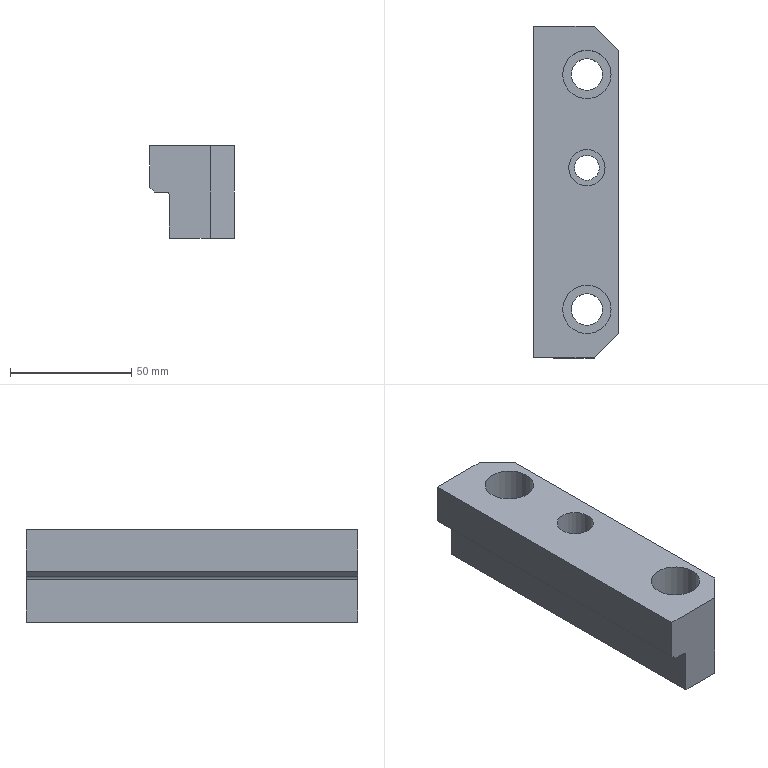Part | STEP file | 1_id598_x_t | 1 solid | 21 faces | box 35 x 137 x 38.1 mm | volume 136243 mm3 | plane 14 | cylinder 7 | commonest cylinder face diameters 13 x2 20 x2 3 x1 10.25 x1 15 x1